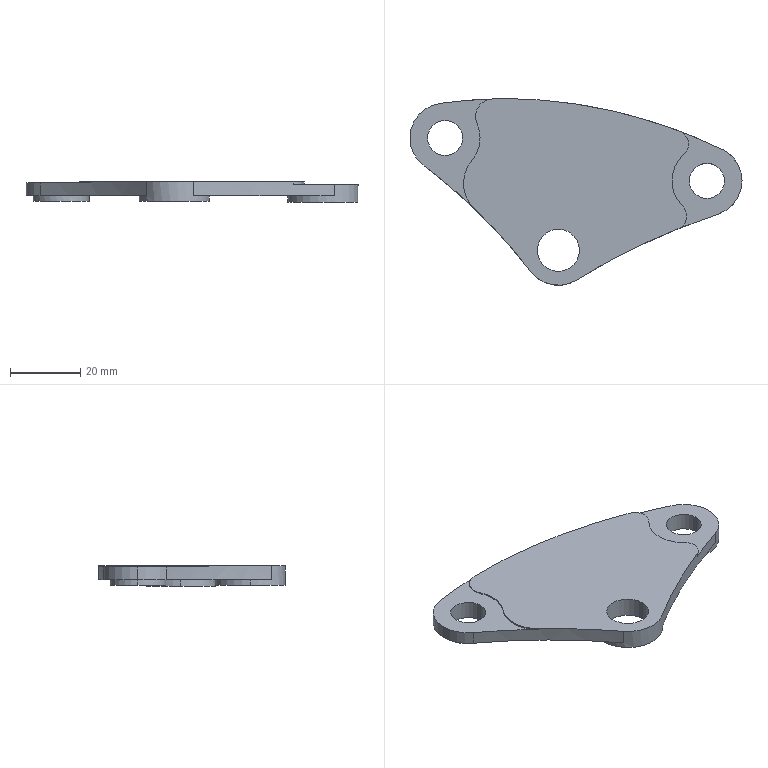Part | NX | features BREP 1 | 1 solid | 49 faces | box 94.779 x 53.231 x 5.8 mm | volume 8618 mm3 | cylinder 37 | plane 8 | spline 4 | commonest cylinder face diameters 20 x11 4 x8 10 x5 8 x4 24 x3 12 x2